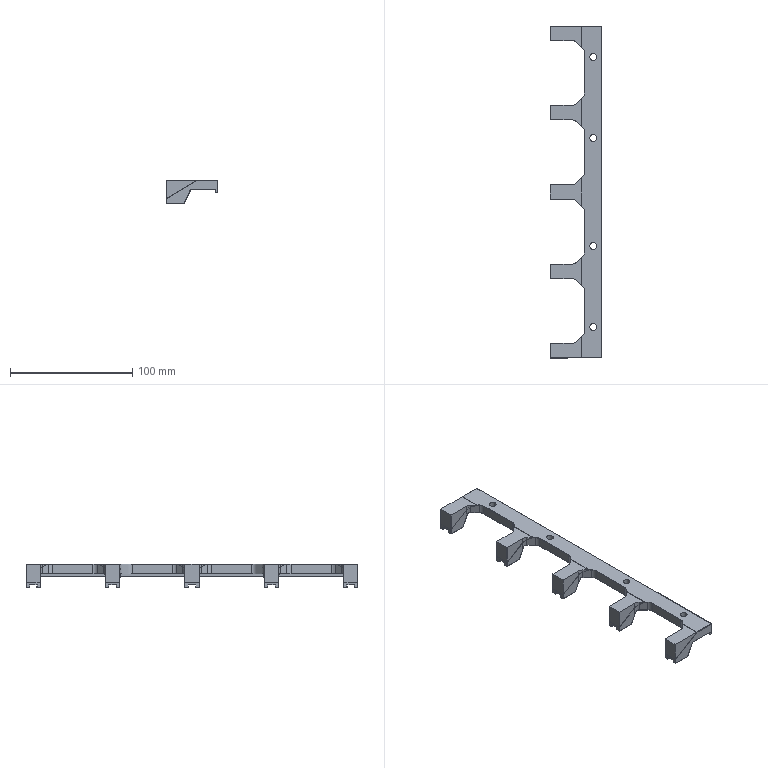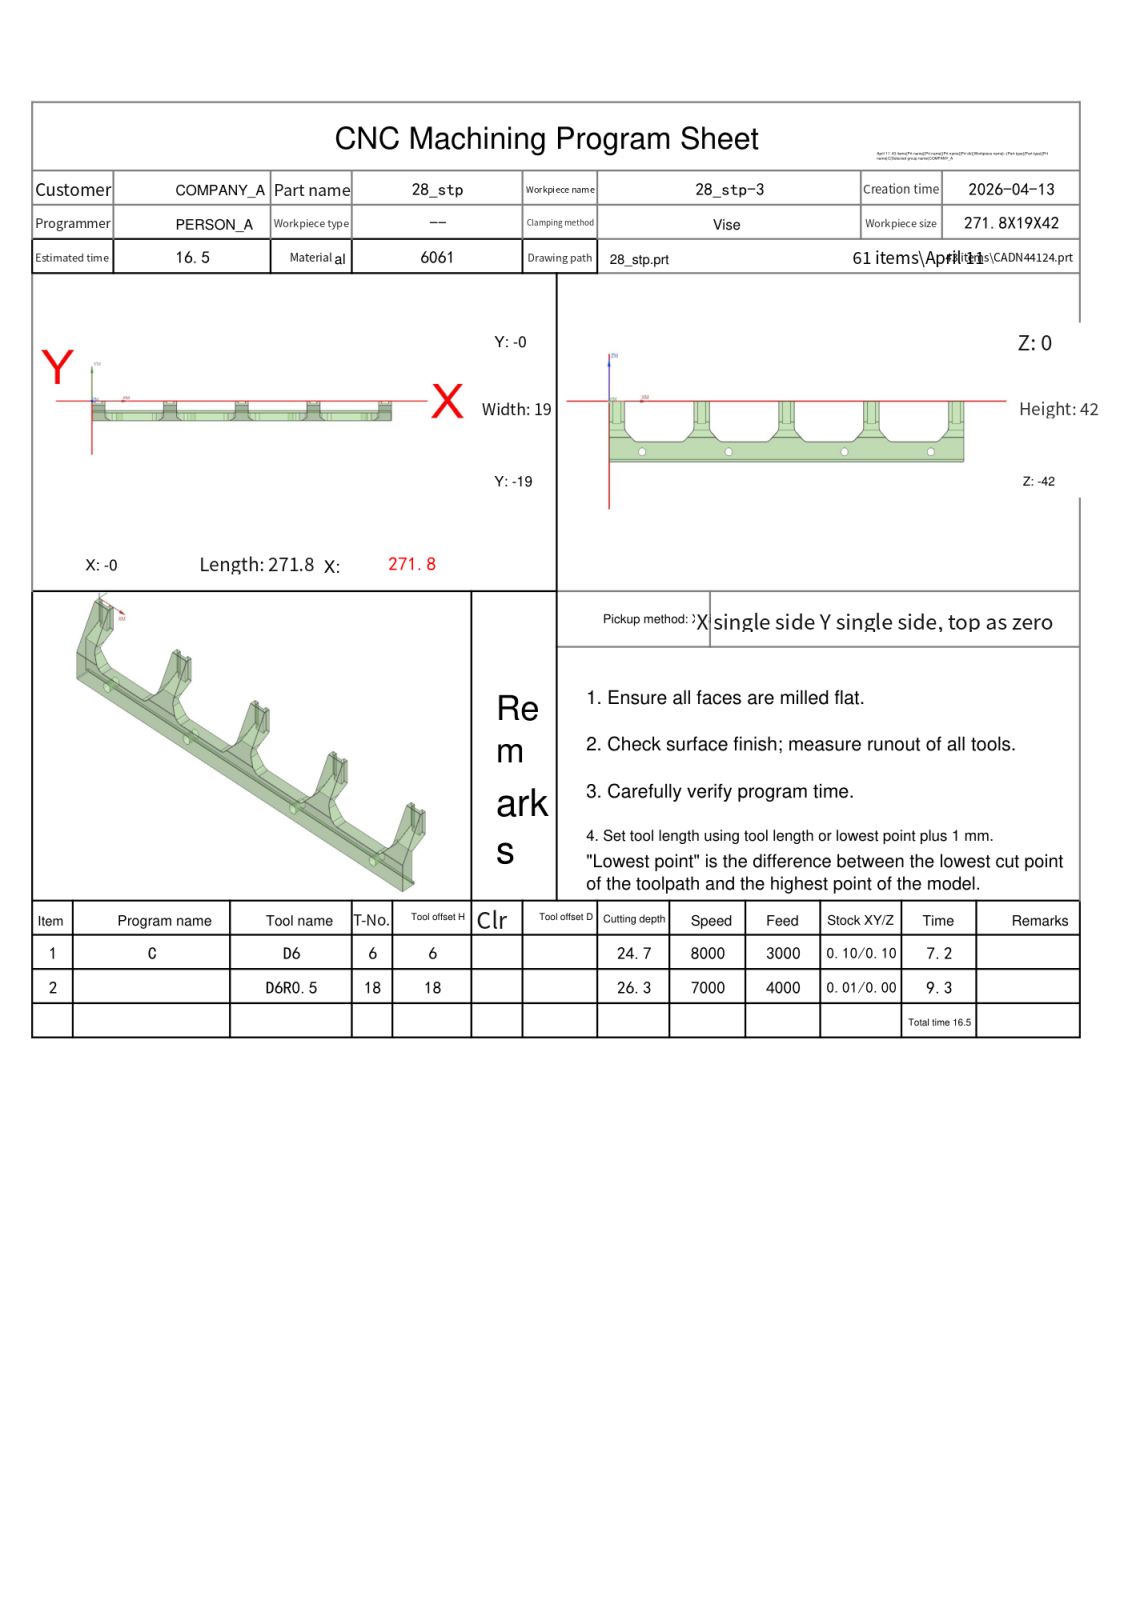NC program | NX | posted by the shop | part box 42 x 271.8 x 19 mm
Lines 1 to 1138 of 25484:
%
O0001
(Machine time: 16.86 MIN)
(===Total Tool:2===)
(T6=D6      D=6.   R=0.   D-  H06 Z=-24.71)
(T18=D6R0.5 D=6.   R=0.5  D-  H18 Z=-26.3 )
G80 G90 G17 G49 G40
G91 G28 Z0
M01
N1 T06 M06
(D6  D=6. R=0. H=06 ce=0.10 di=0.10)
G00 G90 G54 X270.052 Y-26.199 M03 S8000
G43 H06 Z10.1
M08
Z.706
G01 Z-.494 F3000.
Y-23.499
G03 X265.852 Y-19.299 I-4.2 J0.0
G01 X263.805
X261.077
X260.168 Y-19.309
G02 X259.62 Y-18.876 I.045 J.621
G01 X259.605 Y-18.17
X259.603 Y-8.221
G02 X257.471 Y-7.244 I.499 J3.902
G01 X257.47 Y-6.162
X257.549 Y-6.095
X257.752 Y-6.332
G03 X260.1 Y-7.413 I2.35 J2.013
G01 X271.6
G03 X273.948 Y-6.332 I-.002 J3.094
G01 X274.148 Y-6.099
X274.228 Y-6.167
Y-7.245
G02 X272.099 Y-8.221 I-2.63 J2.926
G01 Y-18.166
X272.085 Y-18.789
G02 X271.595 Y-19.28 I-.503 J.012
G01 X270.856 Y-19.299
X262.852
G02 X262.252 Y-18.699 I0.0 J.6
G01 X262.28 Y-18.516
X263.776 Y-13.843
X263.804 Y-13.66
Y-12.211
G02 X264.402 Y-11.613 I.6 J-.002
G01 X267.302
G02 X267.899 Y-12.211 I-.002 J-.6
G01 Y-14.501
G02 X267.302 Y-15.099 I-.6 J.002
G01 X264.402
X264.22 Y-15.07
G02 X263.858 Y-14.746 I.185 J.571
G03 X260.031 Y-12.276 I-3.827 J-1.73
X258.3 Y-12.649 I0.0 J-4.2
G01 X253.272 Y-14.923
Z.706
G00 Z3.
G01 X270.052 Y-26.199 F6000.
G00 Z.212
G01 Z-.988 F3000.
Y-23.499
G03 X265.852 Y-19.299 I-4.2 J0.0
G01 X263.805
X261.077
X260.168 Y-19.309
G02 X259.619 Y-18.875 I.045 J.621
G01 X259.604 Y-18.169
X259.603 Y-8.518
G02 X257.471 Y-7.541 I.499 J3.902
G01 X257.47 Y-6.459
X257.549 Y-6.392
X257.752 Y-6.628
G03 X260.1 Y-7.71 I2.35 J2.013
G01 X271.6
G03 X273.948 Y-6.628 I-.002 J3.094
G01 X274.148 Y-6.395
X274.228 Y-6.464
Y-7.541
G02 X272.099 Y-8.518 I-2.63 J2.926
G01 Y-18.733
G02 X271.534 Y-19.299 I-.566 J0.0
G01 X262.852
G02 X262.252 Y-18.699 I0.0 J.6
G01 X262.28 Y-18.516
X263.775 Y-13.843
X263.804 Y-13.66
X263.803 Y-12.507
G02 X264.401 Y-11.91 I.6 J-.002
G01 X267.302
G02 X267.899 Y-12.507 I-.003 J-.6
G01 Y-14.501
G02 X267.302 Y-15.099 I-.6 J.003
G01 X264.401
X264.219 Y-15.07
G02 X263.857 Y-14.746 I.185 J.571
G03 X260.03 Y-12.277 I-3.827 J-1.731
X258.3 Y-12.65 I0.0 J-4.2
G01 X253.272 Y-14.923
Z.212
G00 Z2.506
G01 X270.051 Y-26.199 F6000.
G00 Z-.282
G01 Z-1.482 F3000.
Y-23.499
G03 X265.851 Y-19.299 I-4.2 J0.0
G01 X263.804
X261.077
X260.168 Y-19.309
G02 X259.619 Y-18.875 I.045 J.621
G01 X259.604 Y-18.168
X259.603 Y-8.814
G02 X257.472 Y-7.837 I.499 J3.902
G01 X257.471 Y-6.754
X257.55 Y-6.689
X257.752 Y-6.925
G03 X260.1 Y-8.006 I2.35 J2.013
G01 X271.6
G03 X273.948 Y-6.925 I-.002 J3.094
G01 X274.148 Y-6.692
X274.228 Y-6.76
Y-7.838
G02 X272.099 Y-8.814 I-2.63 J2.926
G01 Y-18.733
G02 X271.534 Y-19.299 I-.566 J0.0
G01 X262.851
G02 X262.251 Y-18.699 I0.0 J.6
G01 X262.28 Y-18.516
X263.775 Y-13.843
X263.803 Y-13.66
Y-12.803
G02 X264.4 Y-12.206 I.6 J-.003
G01 X267.302
G02 X267.899 Y-12.803 I-.003 J-.6
G01 Y-14.502
G02 X267.302 Y-15.099 I-.6 J.003
G01 X264.401
X264.219 Y-15.07
G02 X263.857 Y-14.746 I.185 J.571
G03 X260.03 Y-12.277 I-3.827 J-1.731
X258.299 Y-12.65 I0.0 J-4.2
G01 X253.272 Y-14.924
Z-.282
G00 Z2.012
G01 X270.051 Y-26.199 F6000.
G00 Z-.776
G01 Z-1.976 F3000.
Y-23.499
G03 X265.851 Y-19.299 I-4.2 J0.0
G01 X263.804
X261.077
X260.168 Y-19.309
G02 X259.619 Y-18.875 I.045 J.621
G01 X259.604 Y-18.168
X259.602 Y-9.111
G02 X257.472 Y-8.134 I.499 J3.902
G01 X257.471 Y-7.054
X257.55 Y-6.986
X257.752 Y-7.221
G03 X260.1 Y-8.303 I2.35 J2.013
G01 X271.6
G03 X273.948 Y-7.221 I-.002 J3.094
G01 X274.148 Y-6.988
X274.228 Y-7.057
Y-8.134
G02 X272.099 Y-9.11 I-2.63 J2.926
G01 Y-18.733
G02 X271.534 Y-19.299 I-.566 J0.0
G01 X262.851
G02 X262.251 Y-18.699 I0.0 J.6
G01 X262.28 Y-18.516
X263.775 Y-13.843
X263.803 Y-13.66
Y-13.099
G02 X264.4 Y-12.503 I.6 J-.003
G01 X267.303
G02 X267.899 Y-13.099 I-.003 J-.6
G01 Y-14.502
G02 X267.303 Y-15.099 I-.6 J.003
G01 X264.4
X264.219 Y-15.07
G02 X263.856 Y-14.746 I.185 J.571
G03 X260.03 Y-12.277 I-3.827 J-1.731
X258.299 Y-12.65 I0.0 J-4.2
G01 X253.272 Y-14.924
Z-.776
G00 Z1.518
G01 X270.051 Y-26.199 F6000.
G00 Z-1.271
G01 Z-2.471 F3000.
Y-23.499
G03 X265.851 Y-19.299 I-4.2 J0.0
G01 X263.804
X261.077
X260.168 Y-19.309
G02 X259.619 Y-18.874 I.045 J.621
G01 X259.603 Y-18.168
X259.602 Y-9.407
G02 X257.472 Y-8.431 I.499 J3.902
G01 X257.471 Y-7.348
X257.551 Y-7.283
X257.752 Y-7.518
G03 X260.1 Y-8.599 I2.35 J2.013
G01 X271.6
G03 X274. Y-7.457 I-.042 J3.181
G01 X274.148 Y-7.284
X274.228 Y-7.353
Y-8.425
G02 X272.099 Y-9.403 I-2.67 J3.007
G01 Y-18.733
G02 X271.534 Y-19.299 I-.566 J0.0
G01 X262.851
G02 X262.251 Y-18.699 I0.0 J.6
G01 X262.28 Y-18.516
X263.774 Y-13.843
X263.803 Y-13.66
Y-13.396
G02 X264.4 Y-12.799 I.6 J-.003
G01 X267.303
G02 X267.899 Y-13.396 I-.003 J-.6
G01 Y-14.502
G02 X267.303 Y-15.099 I-.6 J.003
G01 X264.4
X264.218 Y-15.07
G02 X263.856 Y-14.746 I.185 J.571
G03 X260.03 Y-12.277 I-3.827 J-1.731
X258.299 Y-12.65 I0.0 J-4.2
G01 X253.272 Y-14.924
Z-1.271
G00 Z1.024
G01 X270.051 Y-26.199 F6000.
G00 Z-1.765
G01 Z-2.965 F3000.
Y-23.499
G03 X265.851 Y-19.299 I-4.2 J0.0
G01 X263.803
X261.078
X260.168 Y-19.309
G02 X259.619 Y-18.874 I.045 J.621
G01 X259.603 Y-18.168
X259.602 Y-9.704
G02 X257.472 Y-8.727 I.499 J3.902
G01 Y-8.476
X257.471 Y-7.646
X257.551 Y-7.58
X257.752 Y-7.814
G03 X260.1 Y-8.895 I2.35 J2.013
G01 X271.6
G03 X273.948 Y-7.814 I-.002 J3.094
G01 X274.148 Y-7.581
X274.228 Y-7.65
Y-8.727
G02 X272.099 Y-9.703 I-2.63 J2.926
G01 Y-18.733
G02 X271.534 Y-19.299 I-.566 J0.0
G01 X262.851
G02 X262.251 Y-18.699 I0.0 J.6
G01 X262.28 Y-18.516
X263.775 Y-13.841
X263.803 Y-13.677
G02 X264.399 Y-13.095 I.6 J-.018
G01 X267.303
G02 X267.899 Y-13.692 I-.004 J-.6
G01 Y-14.502
G02 X267.303 Y-15.099 I-.6 J.004
G01 X264.399
X264.218 Y-15.07
G02 X263.856 Y-14.746 I.185 J.571
G03 X260.03 Y-12.277 I-3.827 J-1.731
X258.299 Y-12.65 I0.0 J-4.2
G01 X253.272 Y-14.924
Z-1.765
G00 Z.529
G01 X270.051 Y-26.199 F6000.
G00 Z-2.259
G01 Z-3.459 F3000.
Y-23.499
G03 X265.851 Y-19.299 I-4.2 J0.0
G01 X263.803
X261.078
X260.168 Y-19.309
G02 X259.619 Y-18.874 I.045 J.621
G01 X259.603 Y-18.168
X259.602 Y-10.
G02 X257.472 Y-9.024 I.499 J3.902
G01 Y-8.476
Y-7.943
X257.551 Y-7.877
X257.752 Y-8.111
G03 X260.1 Y-9.192 I2.35 J2.013
G01 X271.6
G03 X274. Y-8.05 I-.042 J3.181
G01 X274.148 Y-7.877
X274.228 Y-7.946
Y-9.018
G02 X272.099 Y-9.996 I-2.67 J3.007
G01 Y-18.733
G02 X271.534 Y-19.299 I-.566 J0.0
G01 X262.851
G02 X262.251 Y-18.699 I0.0 J.6
G01 X262.282 Y-18.508
X263.777 Y-14.063
X263.806 Y-13.932
G02 X264.399 Y-13.392 I.597 J-.06
G01 X267.303
G02 X267.899 Y-13.988 I-.004 J-.6
G01 Y-14.503
G02 X267.303 Y-15.099 I-.6 J.004
G01 X264.399
X264.218 Y-15.07
G02 X263.856 Y-14.746 I.185 J.571
G03 X260.029 Y-12.277 I-3.827 J-1.731
X258.298 Y-12.65 I0.0 J-4.2
G01 X253.272 Y-14.924
Z-2.259
G00 Z.035
G01 X270.051 Y-26.199 F6000.
G00 Z-2.753
G01 Z-3.953 F3000.
Y-23.499
G03 X265.851 Y-19.299 I-4.2 J0.0
G01 X263.803
X261.078
X260.168 Y-19.309
G02 X259.619 Y-18.874 I.045 J.621
G01 X259.603 Y-18.168
X259.602 Y-10.297
G02 X257.472 Y-9.32 I.499 J3.902
G01 Y-8.476
Y-8.242
X257.552 Y-8.174
X257.752 Y-8.407
G03 X260.1 Y-9.488 I2.35 J2.013
G01 X271.6
G03 X274. Y-8.346 I-.042 J3.181
G01 X274.148 Y-8.174
X274.228 Y-8.242
Y-9.314
G02 X272.099 Y-10.292 I-2.67 J3.007
G01 Y-18.733
G02 X271.534 Y-19.299 I-.566 J0.0
G01 X262.851
G02 X262.251 Y-18.699 I0.0 J.6
X262.287 Y-18.496 I.6 J0.0
G01 X263.774 Y-14.364
X263.806 Y-14.225
G02 X264.399 Y-13.688 I.597 J-.064
G01 X267.303
G02 X267.899 Y-14.284 I-.004 J-.6
G01 Y-14.503
G02 X267.303 Y-15.099 I-.6 J.004
G01 X264.399
X264.218 Y-15.07
G02 X263.856 Y-14.746 I.185 J.571
G03 X260.029 Y-12.277 I-3.827 J-1.731
X258.298 Y-12.65 I0.0 J-4.2
G01 X253.272 Y-14.924
Z-2.753
G00 Z-.459
G01 X270.051 Y-26.199 F6000.
G00 Z-3.247
G01 Z-4.447 F3000.
Y-23.499
G03 X265.851 Y-19.299 I-4.2 J0.0
G01 X263.803
X261.078
X260.168 Y-19.309
G02 X259.619 Y-18.874 I.045 J.621
G01 X259.603 Y-18.168
X259.602 Y-10.593
G02 X257.472 Y-9.617 I.5 J3.902
G01 Y-8.539
X257.552 Y-8.471
X257.752 Y-8.704
G03 X260.1 Y-9.785 I2.35 J2.013
G01 X271.6
G03 X273.948 Y-8.704 I-.002 J3.094
G01 X274.148 Y-8.47
X274.228 Y-8.539
Y-9.617
G02 X272.099 Y-10.593 I-2.63 J2.926
G01 Y-18.733
G02 X271.534 Y-19.299 I-.566 J0.0
G01 X262.851
G02 X262.251 Y-18.699 I0.0 J.6
X262.29 Y-18.485 I.6 J0.0
G01 X263.771 Y-14.603
X263.806 Y-14.461
G02 X264.339 Y-13.985 I.536 J-.064
G01 X267.363
G02 X267.901 Y-14.526 I-.004 J-.541
G01 X267.899 Y-14.563
G02 X267.363 Y-15.099 I-.54 J.004
G01 X264.339
X264.181 Y-15.074
G02 X263.834 Y-14.739 I.162 J.515
G03 X259.874 Y-11.94 I-3.96 J-1.401
X258.473 Y-12.18 I0.0 J-4.2
G01 X253.272 Y-14.02
Z-3.247
G00 Z-.953
G01 X270.051 Y-26.199 F6000.
G00 Z-3.741
G01 Z-4.941 F3000.
Y-23.499
G03 X265.851 Y-19.299 I-4.2 J0.0
G01 X263.803
X261.078
X260.168 Y-19.309
G02 X259.619 Y-18.874 I.045 J.621
G01 X259.603 Y-18.168
X259.602 Y-10.889
G02 X257.472 Y-9.913 I.5 J3.902
G01 Y-8.836
X257.552 Y-8.767
X257.752 Y-9.
G03 X260.1 Y-10.081 I2.35 J2.013
G01 X271.6
G03 X273.948 Y-9. I-.002 J3.094
G01 X274.148 Y-8.767
X274.228 Y-8.835
Y-9.913
G02 X272.1 Y-10.889 I-2.63 J2.926
G01 X272.099 Y-18.733
G02 X271.534 Y-19.299 I-.566 J0.0
G01 X262.851
G02 X262.251 Y-18.699 I0.0 J.6
X262.293 Y-18.479 I.6 J0.0
G01 X263.772 Y-14.716
X263.807 Y-14.587
G02 X264.159 Y-14.281 I.356 J-.054
G01 X267.543
G02 X267.899 Y-14.638 I-.003 J-.36
G01 Y-14.742
G02 X267.543 Y-15.099 I-.36 J.003
G01 X264.159
X264.063 Y-15.085
G02 X263.801 Y-14.737 I.1 J.348
G01 X263.803 Y-14.704
G03 X259.603 Y-10.504 I-4.2 J0.0
G01 X253.272 Y-10.505
Z-3.741
G00 Z-1.447
G01 X270.051 Y-26.199 F6000.
G00 Z-4.235
G01 Z-5.435 F3000.
Y-23.499
G03 X265.851 Y-19.299 I-4.2 J0.0
G01 X263.803
X261.078
X260.168 Y-19.309
G02 X259.619 Y-18.874 I.045 J.621
G01 X259.603 Y-18.168
X259.602 Y-11.186
G02 X257.472 Y-10.21 I.5 J3.902
G01 Y-9.132
X257.552 Y-9.063
X257.752 Y-9.296
G03 X260.1 Y-10.378 I2.35 J2.013
G01 X271.6
G03 X274. Y-9.236 I-.042 J3.181
G01 X274.148 Y-9.063
X274.228 Y-9.132
Y-10.204
G02 X272.1 Y-11.181 I-2.67 J3.007
G01 X272.099 Y-18.733
G02 X271.534 Y-19.299 I-.566 J0.0
G01 X262.851
G02 X262.251 Y-18.699 I0.0 J.6
X262.296 Y-18.47 I.6 J0.0
G01 X263.772 Y-14.888
X263.807 Y-14.773
G02 X264.04 Y-14.578 I.236 J-.045
G01 X267.662
G02 X267.903 Y-14.822 I-.004 J-.244
G01 X267.899 Y-14.862
G02 X267.662 Y-15.099 I-.24 J.003
G01 X264.04
X263.98 Y-15.091
G02 X263.799 Y-14.855 I.063 J.236
G01 X263.802 Y-14.815
X263.776 Y-14.733
X263.845 Y-14.682
G03 X264.216 Y-13.49 I-1.729 J1.191
X263.307 Y-11.761 I-2.1 J0.0
G01 X253.272 Y-11.76
Z-4.235
G00 Z-1.941
G01 X270.051 Y-26.199 F6000.
G00 Z-4.729
G01 Z-5.929 F3000.
Y-23.499
G03 X265.851 Y-19.299 I-4.2 J0.0
G01 X262.303
X261.078
X260.168 Y-19.309
G02 X259.618 Y-18.874 I.045 J.621
G01 X259.603 Y-18.168
X259.602 Y-11.482
G02 X257.472 Y-10.506 I.5 J3.902
G01 Y-9.428
X257.552 Y-9.36
X257.752 Y-9.593
G03 X260.1 Y-10.674 I2.35 J2.013
G01 X271.6
G03 X274. Y-9.532 I-.042 J3.181
G01 X274.148 Y-9.36
X274.228 Y-9.428
Y-10.5
G02 X272.1 Y-11.478 I-2.67 J3.007
G01 X272.099 Y-18.733
G02 X271.534 Y-19.299 I-.566 J0.0
G01 X262.851
G02 X262.251 Y-18.699 I0.0 J.6
G01 X262.28 Y-18.516
X262.726 Y-17.12
X262.755 Y-16.938
G03 X262.529 Y-16.468 I-.6 J0.0
G02 X262.302 Y-16.004 I.374 J.469
G01 Y-13.97
G02 X262.898 Y-13.374 I.6 J-.005
G01 X268.804
G02 X269.4 Y-13.97 I-.005 J-.6
G01 X269.399 Y-16.004
G02 X268.804 Y-16.599 I-.6 J.005
G01 X265.851
X262.893
G02 X262.452 Y-16.395 I.009 J.6
G03 X259.3 Y-14.971 I-3.152 J-2.775
X256.524 Y-16.018 I0.0 J-4.2
G01 X252.728 Y-19.361
Z-4.729
G00 Z-2.435
G01 X270.051 Y-26.199 F6000.
G00 Z-5.224
G01 Z-6.424 F3000.
Y-23.499
G03 X265.851 Y-19.299 I-4.2 J0.0
G01 X262.303
X261.078
X260.168 Y-19.309
G02 X259.618 Y-18.874 I.045 J.621
G01 X259.603 Y-18.168
X259.602 Y-11.779
G02 X257.472 Y-10.803 I.5 J3.902
G01 Y-9.725
X257.552 Y-9.656
X257.752 Y-9.889
G03 X260.1 Y-10.971 I2.35 J2.013
G01 X271.601
G03 X273.948 Y-9.889 I-.003 J3.094
G01 X274.148 Y-9.656
X274.228 Y-9.725
Y-10.802
G02 X272.1 Y-11.779 I-2.63 J2.926
G01 X272.099 Y-18.733
G02 X271.534 Y-19.299 I-.565 J0.0
G01 X262.851
G02 X262.251 Y-18.699 I0.0 J.6
G01 X262.279 Y-18.516
X262.726 Y-17.12
X262.755 Y-16.938
G03 X262.529 Y-16.468 I-.6 J0.0
G02 X262.302 Y-16.004 I.374 J.469
G01 Y-14.266
G02 X262.897 Y-13.671 I.6 J-.005
G01 X268.804
G02 X269.4 Y-14.266 I-.005 J-.6
G01 X269.399 Y-16.004
G02 X268.804 Y-16.599 I-.6 J.005
G01 X265.851
X262.893
G02 X262.452 Y-16.395 I.009 J.6
G03 X259.3 Y-14.971 I-3.152 J-2.775
X256.524 Y-16.018 I0.0 J-4.2
G01 X252.728 Y-19.361
Z-5.224
G00 Z-2.929
G01 X270.051 Y-26.199 F6000.
G00 Z-5.718
G01 Z-6.918 F3000.
Y-23.499
G03 X265.851 Y-19.299 I-4.2 J0.0
G01 X262.303
X261.078
X260.168 Y-19.309
G02 X259.618 Y-18.874 I.045 J.621
G01 X259.602 Y-18.167
Y-12.075
G02 X257.472 Y-11.099 I.5 J3.902
G01 Y-10.021
X257.552 Y-9.953
X257.752 Y-10.186
G03 X260.1 Y-11.267 I2.35 J2.013
G01 X271.6
G03 X274.011 Y-10.112 I-.001 J3.096
G01 X274.148 Y-9.953
X274.228 Y-10.021
Y-11.099
G02 X272.1 Y-12.075 I-2.63 J2.926
G01 X272.099 Y-18.733
G02 X271.534 Y-19.299 I-.565 J0.0
G01 X262.851
G02 X262.251 Y-18.699 I0.0 J.6
G01 X262.279 Y-18.516
X262.726 Y-17.12
X262.755 Y-16.938
G03 X262.529 Y-16.468 I-.6 J0.0
G02 X262.302 Y-16.004 I.374 J.469
G01 Y-14.562
G02 X262.897 Y-13.967 I.6 J-.005
G01 X268.805
G02 X269.4 Y-14.562 I-.005 J-.6
G01 Y-16.004
G02 X268.805 Y-16.599 I-.6 J.005
G01 X265.851
X262.893
G02 X262.452 Y-16.395 I.009 J.6
G03 X259.3 Y-14.971 I-3.152 J-2.775
X256.524 Y-16.019 I0.0 J-4.2
G01 X252.728 Y-19.361
Z-5.718
G00 Z-3.424
G01 X270.051 Y-26.199 F6000.
G00 Z-6.212
G01 Z-7.412 F3000.
Y-23.499
G03 X265.851 Y-19.299 I-4.2 J0.0
G01 X262.302
X261.078
X260.168 Y-19.309
G02 X259.618 Y-18.874 I.045 J.621
G01 X259.602 Y-18.167
Y-12.372
G02 X257.472 Y-11.396 I.5 J3.902
G01 Y-10.318
X257.552 Y-10.249
X257.752 Y-10.482
G03 X260.1 Y-11.564 I2.35 J2.013
G01 X271.6
G03 X273.948 Y-10.482 I-.002 J3.094
G01 X274.148 Y-10.249
X274.228 Y-10.318
Y-11.395
G02 X272.1 Y-12.372 I-2.63 J2.926
G01 X272.099 Y-18.734
G02 X271.534 Y-19.299 I-.565 J0.0
G01 X262.851
G02 X262.251 Y-18.699 I0.0 J.6
G01 X262.279 Y-18.516
X262.726 Y-17.12
X262.754 Y-16.938
G03 X262.528 Y-16.468 I-.6 J0.0
G02 X262.302 Y-16.004 I.374 J.469
G01 Y-14.859
G02 X262.897 Y-14.264 I.6 J-.005
G01 X268.805
G02 X269.4 Y-14.858 I-.005 J-.6
G01 Y-16.004
G02 X268.805 Y-16.599 I-.6 J.005
G01 X265.851
X262.893
G02 X262.452 Y-16.395 I.009 J.6
G03 X259.3 Y-14.971 I-3.152 J-2.775
X256.524 Y-16.019 I0.0 J-4.2
G01 X252.727 Y-19.362
Z-6.212
G00 Z-3.918
G01 X270.051 Y-26.199 F6000.
G00 Z-6.706
G01 Z-7.906 F3000.
Y-23.499
G03 X265.851 Y-19.299 I-4.2 J0.0
G01 X262.302
X261.078
X260.167 Y-19.309
G02 X259.618 Y-18.874 I.045 J.621
G01 X259.602 Y-18.167
Y-12.668
G02 X257.472 Y-11.692 I.5 J3.902
G01 Y-10.614
X257.552 Y-10.546
X257.752 Y-10.779
G03 X260.1 Y-11.86 I2.35 J2.013
G01 X271.6
G03 X274. Y-10.718 I-.042 J3.181
G01 X274.148 Y-10.546
X274.228 Y-10.614
Y-11.686
G02 X272.1 Y-12.664 I-2.67 J3.007
G01 X272.099 Y-18.734
G02 X271.534 Y-19.299 I-.565 J0.0
G01 X262.851
G02 X262.251 Y-18.699 I0.0 J.6
G01 X262.279 Y-18.516
X262.726 Y-17.12
X262.754 Y-16.938
G03 X262.528 Y-16.468 I-.6 J0.0
G02 X262.302 Y-16.004 I.374 J.469
G01 Y-15.155
G02 X262.897 Y-14.56 I.6 J-.005
G01 X268.805
G02 X269.4 Y-15.155 I-.005 J-.6
G01 Y-16.004
G02 X268.805 Y-16.599 I-.6 J.005
G01 X265.851
X262.893
G02 X262.452 Y-16.396 I.009 J.6
G03 X259.299 Y-14.971 I-3.152 J-2.776
X256.524 Y-16.019 I0.0 J-4.2
G01 X252.727 Y-19.362
Z-6.706
G00 Z-4.412
G01 X270.051 Y-26.199 F6000.
G00 Z-7.2
G01 Z-8.4 F3000.
Y-23.499
G03 X265.851 Y-19.299 I-4.2 J0.0
G01 X262.302
X261.078
X260.167 Y-19.309
G02 X259.618 Y-18.874 I.045 J.62
G01 X259.602 Y-18.167
Y-12.965
G02 X257.472 Y-11.988 I.5 J3.902
G01 Y-10.911
X257.552 Y-10.842
X257.752 Y-11.075
G03 X260.1 Y-12.157 I2.35 J2.013
G01 X271.6
G03 X274. Y-11.014 I-.042 J3.181
G01 X274.148 Y-10.842
X274.228 Y-10.911
Y-11.983
G02 X272.1 Y-12.96 I-2.67 J3.007
G01 X272.099 Y-18.734
G02 X271.534 Y-19.299 I-.565 J0.0
G01 X262.851
G02 X262.251 Y-18.699 I0.0 J.6
G01 X262.279 Y-18.516
X262.726 Y-17.12
X262.754 Y-16.938
G03 X262.528 Y-16.468 I-.6 J0.0
G02 X262.302 Y-16.005 I.374 J.469
G01 Y-15.451
G02 X262.896 Y-14.857 I.6 J-.005
G01 X268.805
G02 X269.4 Y-15.451 I-.005 J-.6
G01 Y-16.004
G02 X268.805 Y-16.599 I-.6 J.005
G01 X265.851
X262.893
G02 X262.452 Y-16.396 I.009 J.6
G03 X259.299 Y-14.971 I-3.152 J-2.776
X256.524 Y-16.019 I0.0 J-4.2
G01 X252.727 Y-19.362
Z-7.2
G00 Z-4.906
G01 X270.051 Y-26.199 F6000.
G00 Z-7.694
G01 Z-8.894 F3000.
Y-23.499
G03 X265.851 Y-19.299 I-4.2 J0.0
G01 X262.302
X261.078
X260.167 Y-19.309
G02 X259.618 Y-18.874 I.044 J.62
G01 X259.602 Y-18.167
Y-13.261
G02 X257.472 Y-12.285 I.5 J3.902
G01 Y-11.207
X257.552 Y-11.139
X257.752 Y-11.372
G03 X260.1 Y-12.453 I2.35 J2.013
G01 X271.6
G03 X273.948 Y-11.372 I-.002 J3.094
G01 X274.148 Y-11.139
X274.228 Y-11.207
Y-12.285
G02 X272.1 Y-13.261 I-2.63 J2.926
G01 Y-18.734
G02 X271.534 Y-19.299 I-.565 J0.0
G01 X262.851
G02 X262.251 Y-18.699 I0.0 J.6
G01 X262.279 Y-18.516
X262.726 Y-17.12
X262.754 Y-16.938
G03 X262.528 Y-16.468 I-.6 J0.0
G02 X262.302 Y-16.005 I.374 J.469
G01 Y-15.747
G02 X262.896 Y-15.153 I.6 J-.006
G01 X268.805
G02 X269.4 Y-15.747 I-.006 J-.6
G01 Y-16.005
G02 X268.805 Y-16.599 I-.6 J.006
G01 X265.851
X262.892
G02 X262.451 Y-16.396 I.009 J.6
G03 X259.299 Y-14.971 I-3.152 J-2.776
X256.524 Y-16.019 I0.0 J-4.2
G01 X252.727 Y-19.362
Z-7.694
G00 Z-5.4
G01 X270.051 Y-26.199 F6000.
G00 Z-8.188
G01 Z-9.388 F3000.
Y-23.499
G03 X265.851 Y-19.299 I-4.2 J0.0
G01 X262.302
X261.078
X260.167 Y-19.309
G02 X259.618 Y-18.874 I.044 J.62
G01 X259.602 Y-18.167
Y-13.558
G02 X257.472 Y-12.581 I.5 J3.902
G01 Y-11.504
X257.552 Y-11.435
X257.752 Y-11.668
G03 X260.1 Y-12.75 I2.35 J2.013
G01 X271.6
G03 X274. Y-11.607 I-.042 J3.181
G01 X274.148 Y-11.435
X274.228 Y-11.504
Y-12.576
G02 X272.1 Y-13.553 I-2.67 J3.007
G01 Y-18.734
G02 X271.534 Y-19.299 I-.565 J0.0
G01 X262.851
G02 X262.251 Y-18.699 I0.0 J.6
G01 X262.274 Y-18.532
X262.69 Y-17.103
X262.713 Y-16.936
G03 X262.497 Y-16.475 I-.6 J0.0
G02 X262.302 Y-16.065 I.345 J.416
G01 Y-15.984
G02 X262.836 Y-15.45 I.54 J-.005
G01 X268.865
G02 X269.4 Y-15.984 I-.005 J-.54
G01 Y-16.065
G02 X268.865 Y-16.599 I-.54 J.005
G01 X262.851
X262.836
G02 X262.416 Y-16.391 I.005 J.54
G03 X259.101 Y-14.771 I-3.314 J-2.58
X256.521 Y-15.656 I0.0 J-4.2
G01 X252.71 Y-18.623
Z-8.188
G00 Z-5.894
G01 X270.051 Y-26.199 F6000.
G00 Z-8.682
G01 Z-9.882 F3000.
Y-23.499
G03 X265.851 Y-19.299 I-4.2 J0.0
G01 X262.302
X261.078
X260.167 Y-19.309
G02 X259.618 Y-18.874 I.044 J.62
G01 X259.602 Y-18.167
X259.601 Y-13.854
G02 X257.472 Y-12.878 I.5 J3.902
G01 Y-11.8
X257.552 Y-11.732
X257.752 Y-11.965
G03 X260.1 Y-13.046 I2.35 J2.013
G01 X271.6
G03 X273.948 Y-11.965 I-.002 J3.094
G01 X274.148 Y-11.731
X274.228 Y-11.798
Y-12.878
G02 X272.1 Y-13.854 I-2.63 J2.926
G01 Y-18.734
G02 X271.534 Y-19.299 I-.565 J0.0
G01 X262.851
G02 X262.251 Y-18.699 I0.0 J.6
G01 X262.266 Y-18.565
X262.611 Y-17.059
X262.626 Y-16.925
G03 X262.435 Y-16.486 I-.6 J0.0
G02 X262.301 Y-16.179 I.286 J.308
G01 X262.302 Y-16.161
G02 X262.717 Y-15.746 I.42 J-.005
G01 X268.985
G02 X269.4 Y-16.166 I-.005 J-.42
G01 Y-16.184
G02 X268.985 Y-16.599 I-.42 J.005
G01 X262.851
X262.717
G02 X262.397 Y-16.446 I.005 J.42
G03 X259.151 Y-14.911 I-3.246 J-2.665
X256.486 Y-15.865 I0.0 J-4.2
G01 X252.718 Y-18.959
Z-8.682
G00 Z-6.388
G01 X270.051 Y-26.199 F6000.
G00 Z-9.176
G01 Z-10.376 F3000.
Y-23.499
G03 X265.851 Y-19.299 I-4.2 J0.0
G01 X262.302
X261.078
X260.167 Y-19.309
G02 X259.618 Y-18.874 I.044 J.62
G01 X259.602 Y-18.167
X259.601 Y-14.151
G02 X257.472 Y-13.174 I.5 J3.902
G01 Y-12.097
X257.552 Y-12.028
X257.752 Y-12.261
G03 X260.1 Y-13.343 I2.35 J2.013
G01 X271.6
G03 X273.948 Y-12.261 I-.002 J3.094
G01 X274.018 Y-12.179
X274.148 Y-12.028
X274.228 Y-12.095
Y-13.174
G02 X272.1 Y-14.15 I-2.63 J2.926
G01 Y-18.734
G02 X271.534 Y-19.299 I-.565 J0.0
G01 X262.851
G02 X262.251 Y-18.699 I0.0 J.6
G01 X262.256 Y-18.616
X262.485 Y-16.973
X262.491 Y-16.891
G03 X262.356 Y-16.511 I-.6 J0.0
G01 X262.279 Y-16.455
X262.301 Y-16.363
Y-16.279
G02 X262.538 Y-16.043 I.24 J-.004
G01 X269.163
G02 X269.4 Y-16.279 I-.004 J-.24
G01 Y-16.363
G02 X269.163 Y-16.599 I-.24 J.004
G01 X262.851
X262.538
X262.431 Y-16.616
X262.37 Y-16.527
G03 X259.37 Y-15.267 I-3. J-2.94
X256.431 Y-16.467 I0.0 J-4.2
G01 X252.808 Y-20.017
Z-9.176
G00 Z-6.882
G01 X270.05 Y-26.199 F6000.
G00 Z-9.671
G01 Z-10.871 F3000.
Y-23.499
G03 X265.85 Y-19.299 I-4.2 J0.0
G01 X262.302
X261.078
X260.167 Y-19.309
G02 X259.618 Y-18.874 I.044 J.62
G01 X259.601 Y-18.167
Y-14.447
G02 X257.472 Y-13.471 I.5 J3.902
G01 Y-12.393
X257.552 Y-12.324
X257.752 Y-12.558
G03 X260.1 Y-13.639 I2.35 J2.013
G01 X271.6
G03 X273.948 Y-12.558 I-.002 J3.094
G01 X274.148 Y-12.324
X274.228 Y-12.392
Y-13.471
G02 X272.1 Y-14.447 I-2.63 J2.926
G01 Y-18.734
G02 X271.534 Y-19.299 I-.565 J0.0
G01 X262.85
G02 X262.25 Y-18.699 I0.0 J.6
G01 X262.252 Y-18.651
X262.395 Y-16.888
X262.397 Y-16.839
G03 X262.316 Y-16.538 I-.6 J0.0
G01 X262.301 Y-16.456
X262.283 Y-16.378
X262.34 Y-16.321
X262.419 Y-16.339
X269.282
X269.401 Y-16.461
X269.4 Y-16.482
X269.418 Y-16.56
X269.361 Y-16.617
X269.282 Y-16.599
X262.85
X262.419
X262.355 Y-16.579
G03 X260.016 Y-15.867 I-2.339 J-3.489
X256.527 Y-17.729 I0.0 J-4.2
G01 X253.546 Y-22.175
Z-9.671
G00 Z-7.376
G01 X270.051 Y-26.199 F6000.
G00 Z-10.165
G01 Z-11.365 F3000.
Y-23.499
G03 X265.851 Y-19.299 I-4.2 J0.0
G01 X261.078
X260.167 Y-19.309
G02 X259.618 Y-18.874 I.044 J.62
G01 X259.601 Y-18.167
Y-14.743
G02 X257.472 Y-13.767 I.501 J3.902
G01 Y-12.69
X257.552 Y-12.621
X257.752 Y-12.854
G03 X260.1 Y-13.935 I2.35 J2.013
G01 X271.6
G03 X273.948 Y-12.854 I-.002 J3.094
G01 X274.148 Y-12.621
X274.228 Y-12.69
Y-13.767
G02 X272.1 Y-14.743 I-2.63 J2.926
G01 Y-18.734
G02 X271.534 Y-19.299 I-.565 J0.0
G01 X265.851
X265.351
G03 X261.151 Y-23.499 I0.0 J-4.2
G01 Y-26.199
Z-10.165
G00 Z-7.871
G01 X270.051 F6000.
G00 Z-10.659
G01 Z-11.859 F3000.
Y-23.499
G03 X265.851 Y-19.299 I-4.2 J0.0
G01 X261.078
X260.167 Y-19.309
G02 X259.618 Y-18.874 I.044 J.62
G01 X259.601 Y-18.167
Y-15.04
G02 X257.472 Y-14.064 I.501 J3.902
G01 Y-12.986
X257.552 Y-12.917
X257.752 Y-13.151
G03 X260.1 Y-14.232 I2.35 J2.012
G01 X271.6
G03 X274. Y-13.09 I-.042 J3.181
G01 X274.148 Y-12.917
X274.228 Y-12.986
Y-14.058
G02 X272.1 Y-15.036 I-2.67 J3.007
G01 Y-18.734
G02 X271.534 Y-19.299 I-.565 J0.0
G01 X265.851
X265.351
G03 X261.151 Y-23.499 I0.0 J-4.2
G01 Y-26.199
Z-10.659
G00 Z-8.365
G01 X270.051 F6000.
G00 Z-11.153
G01 Z-12.353 F3000.
Y-23.499
G03 X265.851 Y-19.299 I-4.2 J0.0
G01 X261.078
X260.167 Y-19.309
G02 X259.617 Y-18.874 I.044 J.62
G01 X259.601 Y-18.167
Y-15.336
G02 X257.472 Y-14.36 I.501 J3.902
G01 Y-13.282
X257.552 Y-13.214
X257.752 Y-13.447
G03 X260.1 Y-14.528 I2.35 J2.012
G01 X271.6
G03 X273.948 Y-13.447 I-.002 J3.094
G01 X274.148 Y-13.214
X274.228 Y-13.282
Y-14.36
G02 X272.1 Y-15.336 I-2.63 J2.926
G01 Y-18.734
G02 X271.534 Y-19.299 I-.565 J0.0
G01 X265.851
X265.351
G03 X261.151 Y-23.499 I0.0 J-4.2
G01 Y-26.199
Z-11.153
G00 Z-8.859
G01 X270.051 F6000.
G00 Z-11.647
G01 Z-12.847 F3000.
Y-23.499
G03 X265.851 Y-19.299 I-4.2 J0.0
G01 X261.078
X260.167 Y-19.309
G02 X259.617 Y-18.874 I.044 J.62
G01 X259.601 Y-18.167
Y-15.633
G02 X257.472 Y-14.657 I.501 J3.902
G01 Y-13.579
X257.552 Y-13.51
X257.752 Y-13.744
G03 X260.1 Y-14.825 I2.35 J2.012
G01 X271.6
G03 X274. Y-13.683 I-.042 J3.181
G01 X274.148 Y-13.51
X274.228 Y-13.579
Y-14.651
G02 X272.1 Y-15.629 I-2.67 J3.007
G01 Y-18.734
G02 X271.534 Y-19.299 I-.565 J0.0
G01 X265.851
X265.351
G03 X261.151 Y-23.499 I0.0 J-4.2
G01 Y-26.199
Z-11.647
G00 Z-9.353
G01 X270.051 F6000.
G00 Z-12.141
G01 Z-13.341 F3000.
Y-23.499
G03 X265.851 Y-19.299 I-4.2 J0.0
G01 X261.078
X260.167 Y-19.309
G02 X259.617 Y-18.874 I.044 J.62
G01 X259.601 Y-18.167
Y-15.929
G02 X257.472 Y-14.953 I.501 J3.902
G01 Y-13.875
X257.552 Y-13.807
X257.752 Y-14.04
G03 X260.1 Y-15.121 I2.35 J2.012
G01 X271.6
G03 X273.948 Y-14.04 I-.002 J3.094
G01 X274.148 Y-13.807
X274.228 Y-13.875
Y-14.953
G02 X272.1 Y-15.929 I-2.63 J2.926
G01 Y-18.734
G02 X271.534 Y-19.299 I-.565 J0.0
G01 X265.851
X265.351
G03 X261.151 Y-23.499 I0.0 J-4.2
G01 Y-26.199
Z-12.141
G00 Z-9.847
G01 X270.051 F6000.
G00 Z-12.635